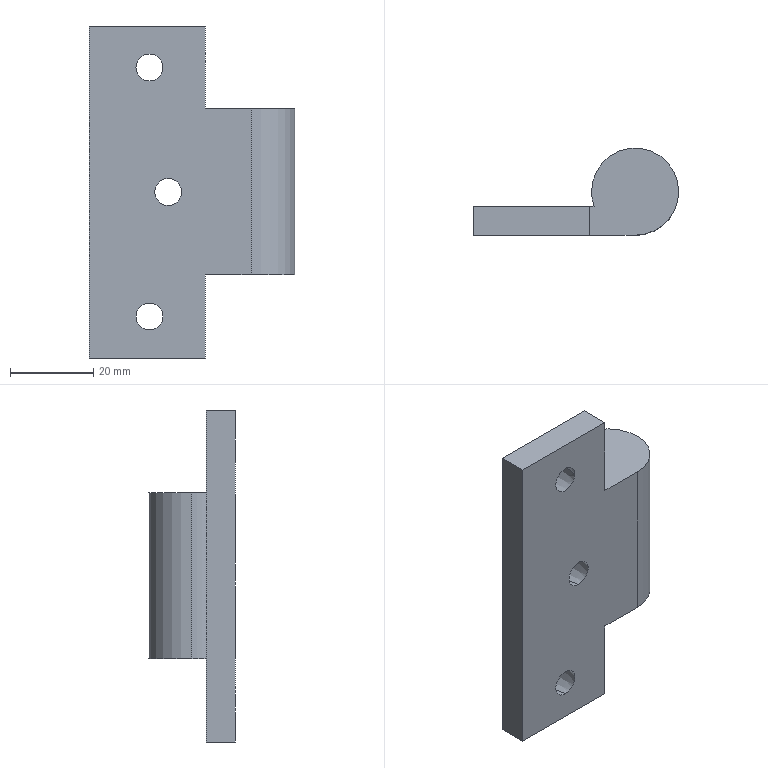Part | SolidWorks | features BaseBody 1 | 1 solid | 18 faces | box 49.5 x 21 x 80 mm | volume 29616 mm3 | plane 9 | cone 6 | cylinder 3 | commonest cylinder face diameters 21 x3
STEP:
#1=CARTESIAN_POINT('',(-10.5,0.,-20.));
#2=VERTEX_POINT('',#1);
#3=CARTESIAN_POINT('',(10.5,0.,-20.));
#4=VERTEX_POINT('',#3);
#5=CARTESIAN_POINT('',(0.,0.,-20.));
#6=DIRECTION('',(0.,0.,-1.));
#7=DIRECTION('',(1.,0.,0.));
#8=AXIS2_PLACEMENT_3D('',#5,#6,#7);
#9=CIRCLE('',#8,10.5);
#10=EDGE_CURVE('',#2,#4,#9,.T.);
#11=ORIENTED_EDGE('',*,*,#10,.F.);
#12=CARTESIAN_POINT('',(-10.5,0.,20.));
#13=VERTEX_POINT('',#12);
#14=CARTESIAN_POINT('',(-10.5,0.,40.));
#15=DIRECTION('',(0.,0.,1.));
#16=VECTOR('',#15,1000.);
#17=LINE('',#14,#16);
#18=EDGE_CURVE('',#2,#13,#17,.T.);
#19=ORIENTED_EDGE('',*,*,#18,.T.);
#20=CARTESIAN_POINT('',(10.5,0.,20.));
#21=VERTEX_POINT('',#20);
#22=CARTESIAN_POINT('',(0.,0.,20.));
#23=DIRECTION('',(0.,0.,1.));
#24=DIRECTION('',(1.,0.,0.));
#25=AXIS2_PLACEMENT_3D('',#22,#23,#24);
#26=CIRCLE('',#25,10.5);
#27=EDGE_CURVE('',#21,#13,#26,.T.);
#28=ORIENTED_EDGE('',*,*,#27,.F.);
#29=CARTESIAN_POINT('',(10.5,0.,40.));
#30=DIRECTION('',(0.,0.,1.));
#31=VECTOR('',#30,1000.);
#32=LINE('',#29,#31);
#33=EDGE_CURVE('',#4,#21,#32,.T.);
#34=ORIENTED_EDGE('',*,*,#33,.F.);
#35=EDGE_LOOP('',(#11,#19,#28,#34));
#36=FACE_OUTER_BOUND('',#35,.T.);
#37=CARTESIAN_POINT('',(0.,0.,40.));
#38=DIRECTION('',(0.,0.,1.));
#39=DIRECTION('',(1.,0.,0.));
#40=AXIS2_PLACEMENT_3D('',#37,#38,#39);
#41=CYLINDRICAL_SURFACE('',#40,10.5);
#42=ADVANCED_FACE('',(#36),#41,.T.);
#43=CARTESIAN_POINT('',(0.,-10.5,-20.));
#44=VERTEX_POINT('',#43);
#45=CARTESIAN_POINT('',(0.,0.,-20.));
#46=DIRECTION('',(0.,0.,-1.));
#47=DIRECTION('',(1.,0.,0.));
#48=AXIS2_PLACEMENT_3D('',#45,#46,#47);
#49=CIRCLE('',#48,10.5);
#50=EDGE_CURVE('',#4,#44,#49,.T.);
#51=ORIENTED_EDGE('',*,*,#50,.F.);
#52=ORIENTED_EDGE('',*,*,#33,.T.);
#53=CARTESIAN_POINT('',(0.,-10.5,20.));
#54=VERTEX_POINT('',#53);
#55=CARTESIAN_POINT('',(0.,0.,20.));
#56=DIRECTION('',(0.,0.,1.));
#57=DIRECTION('',(1.,0.,0.));
#58=AXIS2_PLACEMENT_3D('',#55,#56,#57);
#59=CIRCLE('',#58,10.5);
#60=EDGE_CURVE('',#54,#21,#59,.T.);
#61=ORIENTED_EDGE('',*,*,#60,.F.);
#62=CARTESIAN_POINT('',(0.,-10.5,40.));
#63=DIRECTION('',(0.,0.,-1.));
#64=VECTOR('',#63,1000.);
#65=LINE('',#62,#64);
#66=EDGE_CURVE('',#54,#44,#65,.T.);
#67=ORIENTED_EDGE('',*,*,#66,.T.);
#68=EDGE_LOOP('',(#51,#52,#61,#67));
#69=FACE_OUTER_BOUND('',#68,.T.);
#70=CARTESIAN_POINT('',(0.,0.,40.));
#71=DIRECTION('',(0.,0.,1.));
#72=DIRECTION('',(1.,0.,0.));
#73=AXIS2_PLACEMENT_3D('',#70,#71,#72);
#74=CYLINDRICAL_SURFACE('',#73,10.5);
#75=ADVANCED_FACE('',(#69),#74,.T.);
#76=CARTESIAN_POINT('',(-20.,-10.5,3.25));
#77=VERTEX_POINT('',#76);
#78=CARTESIAN_POINT('',(-20.,-10.5,-3.25));
#79=VERTEX_POINT('',#78);
#80=CARTESIAN_POINT('',(-20.,-10.5,0.));
#81=DIRECTION('',(0.,-1.,0.));
#82=DIRECTION('',(0.,0.,1.));
#83=AXIS2_PLACEMENT_3D('',#80,#81,#82);
#84=CIRCLE('',#83,3.25);
#85=EDGE_CURVE('',#77,#79,#84,.T.);
#86=ORIENTED_EDGE('',*,*,#85,.T.);
#87=CARTESIAN_POINT('',(-20.,-3.5,-4.417));
#88=VERTEX_POINT('',#87);
#89=CARTESIAN_POINT('',(-20.,-3.5,-4.417));
#90=DIRECTION('',(0.,0.9864,-0.1644));
#91=VECTOR('',#90,1000.);
#92=LINE('',#89,#91);
#93=EDGE_CURVE('',#79,#88,#92,.T.);
#94=ORIENTED_EDGE('',*,*,#93,.T.);
#95=CARTESIAN_POINT('',(-20.,-3.5,4.417));
#96=VERTEX_POINT('',#95);
#97=CARTESIAN_POINT('',(-20.,-3.5,0.));
#98=DIRECTION('',(0.,-1.,0.));
#99=DIRECTION('',(0.,0.,1.));
#100=AXIS2_PLACEMENT_3D('',#97,#98,#99);
#101=CIRCLE('',#100,4.417);
#102=EDGE_CURVE('',#96,#88,#101,.T.);
#103=ORIENTED_EDGE('',*,*,#102,.F.);
#104=CARTESIAN_POINT('',(-20.,-3.5,4.417));
#105=DIRECTION('',(0.,0.9864,0.1644));
#106=VECTOR('',#105,1000.);
#107=LINE('',#104,#106);
#108=EDGE_CURVE('',#77,#96,#107,.T.);
#109=ORIENTED_EDGE('',*,*,#108,.F.);
#110=EDGE_LOOP('',(#86,#94,#103,#109));
#111=FACE_OUTER_BOUND('',#110,.T.);
#112=CARTESIAN_POINT('',(-20.,-3.5,0.));
#113=DIRECTION('',(0.,1.,0.));
#114=DIRECTION('',(0.,0.,1.));
#115=AXIS2_PLACEMENT_3D('',#112,#113,#114);
#116=CONICAL_SURFACE('',#115,4.417,0.1651);
#117=ADVANCED_FACE('',(#111),#116,.F.);
#118=CARTESIAN_POINT('',(-24.5,-10.5,-26.75));
#119=VERTEX_POINT('',#118);
#120=CARTESIAN_POINT('',(-24.5,-10.5,-33.25));
#121=VERTEX_POINT('',#120);
#122=CARTESIAN_POINT('',(-24.5,-10.5,-30.));
#123=DIRECTION('',(0.,-1.,0.));
#124=DIRECTION('',(0.,0.,1.));
#125=AXIS2_PLACEMENT_3D('',#122,#123,#124);
#126=CIRCLE('',#125,3.25);
#127=EDGE_CURVE('',#119,#121,#126,.T.);
#128=ORIENTED_EDGE('',*,*,#127,.T.);
#129=CARTESIAN_POINT('',(-24.5,-3.5,-34.417));
#130=VERTEX_POINT('',#129);
#131=CARTESIAN_POINT('',(-24.5,-3.5,-34.417));
#132=DIRECTION('',(0.,0.9864,-0.1644));
#133=VECTOR('',#132,1000.);
#134=LINE('',#131,#133);
#135=EDGE_CURVE('',#121,#130,#134,.T.);
#136=ORIENTED_EDGE('',*,*,#135,.T.);
#137=CARTESIAN_POINT('',(-24.5,-3.5,-25.583));
#138=VERTEX_POINT('',#137);
#139=CARTESIAN_POINT('',(-24.5,-3.5,-30.));
#140=DIRECTION('',(0.,-1.,0.));
#141=DIRECTION('',(0.,0.,1.));
#142=AXIS2_PLACEMENT_3D('',#139,#140,#141);
#143=CIRCLE('',#142,4.417);
#144=EDGE_CURVE('',#138,#130,#143,.T.);
#145=ORIENTED_EDGE('',*,*,#144,.F.);
#146=CARTESIAN_POINT('',(-24.5,-3.5,-25.583));
#147=DIRECTION('',(0.,0.9864,0.1644));
#148=VECTOR('',#147,1000.);
#149=LINE('',#146,#148);
#150=EDGE_CURVE('',#119,#138,#149,.T.);
#151=ORIENTED_EDGE('',*,*,#150,.F.);
#152=EDGE_LOOP('',(#128,#136,#145,#151));
#153=FACE_OUTER_BOUND('',#152,.T.);
#154=CARTESIAN_POINT('',(-24.5,-3.5,-30.));
#155=DIRECTION('',(0.,1.,0.));
#156=DIRECTION('',(0.,0.,1.));
#157=AXIS2_PLACEMENT_3D('',#154,#155,#156);
#158=CONICAL_SURFACE('',#157,4.417,0.1651);
#159=ADVANCED_FACE('',(#153),#158,.F.);
#160=CARTESIAN_POINT('',(-27.75,-10.5,30.));
#161=VERTEX_POINT('',#160);
#162=CARTESIAN_POINT('',(-21.25,-10.5,30.));
#163=VERTEX_POINT('',#162);
#164=CARTESIAN_POINT('',(-24.5,-10.5,30.));
#165=DIRECTION('',(0.,-1.,0.));
#166=DIRECTION('',(-1.,0.,0.));
#167=AXIS2_PLACEMENT_3D('',#164,#165,#166);
#168=CIRCLE('',#167,3.25);
#169=EDGE_CURVE('',#161,#163,#168,.T.);
#170=ORIENTED_EDGE('',*,*,#169,.T.);
#171=CARTESIAN_POINT('',(-20.083,-3.5,30.));
#172=VERTEX_POINT('',#171);
#173=CARTESIAN_POINT('',(-20.083,-3.5,30.));
#174=DIRECTION('',(0.1644,0.9864,0.));
#175=VECTOR('',#174,1000.);
#176=LINE('',#173,#175);
#177=EDGE_CURVE('',#163,#172,#176,.T.);
#178=ORIENTED_EDGE('',*,*,#177,.T.);
#179=CARTESIAN_POINT('',(-28.917,-3.5,30.));
#180=VERTEX_POINT('',#179);
#181=CARTESIAN_POINT('',(-24.5,-3.5,30.));
#182=DIRECTION('',(0.,-1.,0.));
#183=DIRECTION('',(-1.,0.,0.));
#184=AXIS2_PLACEMENT_3D('',#181,#182,#183);
#185=CIRCLE('',#184,4.417);
#186=EDGE_CURVE('',#180,#172,#185,.T.);
#187=ORIENTED_EDGE('',*,*,#186,.F.);
#188=CARTESIAN_POINT('',(-28.917,-3.5,30.));
#189=DIRECTION('',(-0.1644,0.9864,0.));
#190=VECTOR('',#189,1000.);
#191=LINE('',#188,#190);
#192=EDGE_CURVE('',#161,#180,#191,.T.);
#193=ORIENTED_EDGE('',*,*,#192,.F.);
#194=EDGE_LOOP('',(#170,#178,#187,#193));
#195=FACE_OUTER_BOUND('',#194,.T.);
#196=CARTESIAN_POINT('',(-24.5,-3.5,30.));
#197=DIRECTION('',(0.,1.,0.));
#198=DIRECTION('',(-1.,0.,0.));
#199=AXIS2_PLACEMENT_3D('',#196,#197,#198);
#200=CONICAL_SURFACE('',#199,4.417,0.1651);
#201=ADVANCED_FACE('',(#195),#200,.F.);
#202=CARTESIAN_POINT('',(-11.,-10.5,40.));
#203=VERTEX_POINT('',#202);
#204=CARTESIAN_POINT('',(-11.,-10.5,20.));
#205=VERTEX_POINT('',#204);
#206=CARTESIAN_POINT('',(-11.,-10.5,40.));
#207=DIRECTION('',(0.,0.,-1.));
#208=VECTOR('',#207,1000.);
#209=LINE('',#206,#208);
#210=EDGE_CURVE('',#203,#205,#209,.T.);
#211=ORIENTED_EDGE('',*,*,#210,.F.);
#212=CARTESIAN_POINT('',(-39.,-10.5,40.));
#213=VERTEX_POINT('',#212);
#214=CARTESIAN_POINT('',(-39.,-10.5,40.));
#215=DIRECTION('',(1.,0.,0.));
#216=VECTOR('',#215,1000.);
#217=LINE('',#214,#216);
#218=EDGE_CURVE('',#213,#203,#217,.T.);
#219=ORIENTED_EDGE('',*,*,#218,.F.);
#220=CARTESIAN_POINT('',(-39.,-10.5,-40.));
#221=VERTEX_POINT('',#220);
#222=CARTESIAN_POINT('',(-39.,-10.5,40.));
#223=DIRECTION('',(0.,0.,1.));
#224=VECTOR('',#223,1000.);
#225=LINE('',#222,#224);
#226=EDGE_CURVE('',#221,#213,#225,.T.);
#227=ORIENTED_EDGE('',*,*,#226,.F.);
#228=CARTESIAN_POINT('',(-11.,-10.5,-40.));
#229=VERTEX_POINT('',#228);
#230=CARTESIAN_POINT('',(-39.,-10.5,-40.));
#231=DIRECTION('',(-1.,0.,0.));
#232=VECTOR('',#231,1000.);
#233=LINE('',#230,#232);
#234=EDGE_CURVE('',#229,#221,#233,.T.);
#235=ORIENTED_EDGE('',*,*,#234,.F.);
#236=CARTESIAN_POINT('',(-11.,-10.5,-20.));
#237=VERTEX_POINT('',#236);
#238=CARTESIAN_POINT('',(-11.,-10.5,40.));
#239=DIRECTION('',(0.,0.,-1.));
#240=VECTOR('',#239,1000.);
#241=LINE('',#238,#240);
#242=EDGE_CURVE('',#237,#229,#241,.T.);
#243=ORIENTED_EDGE('',*,*,#242,.F.);
#244=CARTESIAN_POINT('',(-39.,-10.5,-20.));
#245=DIRECTION('',(-1.,0.,0.));
#246=VECTOR('',#245,1000.);
#247=LINE('',#244,#246);
#248=EDGE_CURVE('',#44,#237,#247,.T.);
#249=ORIENTED_EDGE('',*,*,#248,.F.);
#250=ORIENTED_EDGE('',*,*,#66,.F.);
#251=CARTESIAN_POINT('',(-39.,-10.5,20.));
#252=DIRECTION('',(1.,0.,0.));
#253=VECTOR('',#252,1000.);
#254=LINE('',#251,#253);
#255=EDGE_CURVE('',#205,#54,#254,.T.);
#256=ORIENTED_EDGE('',*,*,#255,.F.);
#257=EDGE_LOOP('',(#211,#219,#227,#235,#243,#249,#250,#256));
#258=FACE_OUTER_BOUND('',#257,.T.);
#259=ORIENTED_EDGE('',*,*,#85,.F.);
#260=CARTESIAN_POINT('',(-20.,-10.5,0.));
#261=DIRECTION('',(0.,-1.,0.));
#262=DIRECTION('',(0.,0.,1.));
#263=AXIS2_PLACEMENT_3D('',#260,#261,#262);
#264=CIRCLE('',#263,3.25);
#265=EDGE_CURVE('',#79,#77,#264,.T.);
#266=ORIENTED_EDGE('',*,*,#265,.F.);
#267=EDGE_LOOP('',(#259,#266));
#268=FACE_BOUND('',#267,.T.);
#269=ORIENTED_EDGE('',*,*,#127,.F.);
#270=CARTESIAN_POINT('',(-24.5,-10.5,-30.));
#271=DIRECTION('',(0.,-1.,0.));
#272=DIRECTION('',(0.,0.,1.));
#273=AXIS2_PLACEMENT_3D('',#270,#271,#272);
#274=CIRCLE('',#273,3.25);
#275=EDGE_CURVE('',#121,#119,#274,.T.);
#276=ORIENTED_EDGE('',*,*,#275,.F.);
#277=EDGE_LOOP('',(#269,#276));
#278=FACE_BOUND('',#277,.T.);
#279=ORIENTED_EDGE('',*,*,#169,.F.);
#280=CARTESIAN_POINT('',(-24.5,-10.5,30.));
#281=DIRECTION('',(0.,-1.,0.));
#282=DIRECTION('',(-1.,0.,0.));
#283=AXIS2_PLACEMENT_3D('',#280,#281,#282);
#284=CIRCLE('',#283,3.25);
#285=EDGE_CURVE('',#163,#161,#284,.T.);
#286=ORIENTED_EDGE('',*,*,#285,.F.);
#287=EDGE_LOOP('',(#279,#286));
#288=FACE_BOUND('',#287,.T.);
#289=CARTESIAN_POINT('',(-39.,-10.5,40.));
#290=DIRECTION('',(0.,1.,0.));
#291=DIRECTION('',(0.,0.,1.));
#292=AXIS2_PLACEMENT_3D('',#289,#290,#291);
#293=PLANE('',#292);
#294=ADVANCED_FACE('',(#258,#268,#278,#288),#293,.F.);
#295=ORIENTED_EDGE('',*,*,#255,.T.);
#296=ORIENTED_EDGE('',*,*,#60,.T.);
#297=ORIENTED_EDGE('',*,*,#27,.T.);
#298=CARTESIAN_POINT('',(-9.899,-3.5,20.));
#299=VERTEX_POINT('',#298);
#300=CARTESIAN_POINT('',(0.,0.,20.));
#301=DIRECTION('',(0.,0.,1.));
#302=DIRECTION('',(1.,0.,0.));
#303=AXIS2_PLACEMENT_3D('',#300,#301,#302);
#304=CIRCLE('',#303,10.5);
#305=EDGE_CURVE('',#13,#299,#304,.T.);
#306=ORIENTED_EDGE('',*,*,#305,.T.);
#307=CARTESIAN_POINT('',(-11.,-3.5,20.));
#308=VERTEX_POINT('',#307);
#309=CARTESIAN_POINT('',(-9.899,-3.5,20.));
#310=DIRECTION('',(-1.,0.,0.));
#311=VECTOR('',#310,1000.);
#312=LINE('',#309,#311);
#313=EDGE_CURVE('',#299,#308,#312,.T.);
#314=ORIENTED_EDGE('',*,*,#313,.T.);
#315=CARTESIAN_POINT('',(-11.,19.,20.));
#316=DIRECTION('',(0.,-1.,0.));
#317=VECTOR('',#316,1000.);
#318=LINE('',#315,#317);
#319=EDGE_CURVE('',#308,#205,#318,.T.);
#320=ORIENTED_EDGE('',*,*,#319,.T.);
#321=EDGE_LOOP('',(#295,#296,#297,#306,#314,#320));
#322=FACE_OUTER_BOUND('',#321,.T.);
#323=CARTESIAN_POINT('',(11.,19.,20.));
#324=DIRECTION('',(0.,0.,1.));
#325=DIRECTION('',(1.,0.,0.));
#326=AXIS2_PLACEMENT_3D('',#323,#324,#325);
#327=PLANE('',#326);
#328=ADVANCED_FACE('',(#322),#327,.T.);
#329=ORIENTED_EDGE('',*,*,#210,.T.);
#330=ORIENTED_EDGE('',*,*,#319,.F.);
#331=CARTESIAN_POINT('',(-11.,-3.5,40.));
#332=VERTEX_POINT('',#331);
#333=CARTESIAN_POINT('',(-11.,-3.5,20.));
#334=DIRECTION('',(0.,0.,1.));
#335=VECTOR('',#334,1000.);
#336=LINE('',#333,#335);
#337=EDGE_CURVE('',#308,#332,#336,.T.);
#338=ORIENTED_EDGE('',*,*,#337,.T.);
#339=CARTESIAN_POINT('',(-11.,19.,40.));
#340=DIRECTION('',(0.,-1.,0.));
#341=VECTOR('',#340,1000.);
#342=LINE('',#339,#341);
#343=EDGE_CURVE('',#332,#203,#342,.T.);
#344=ORIENTED_EDGE('',*,*,#343,.T.);
#345=EDGE_LOOP('',(#329,#330,#338,#344));
#346=FACE_OUTER_BOUND('',#345,.T.);
#347=CARTESIAN_POINT('',(-11.,19.,20.));
#348=DIRECTION('',(1.,0.,0.));
#349=DIRECTION('',(0.,0.,-1.));
#350=AXIS2_PLACEMENT_3D('',#347,#348,#349);
#351=PLANE('',#350);
#352=ADVANCED_FACE('',(#346),#351,.T.);
#353=CARTESIAN_POINT('',(-39.,-3.5,40.));
#354=VERTEX_POINT('',#353);
#355=CARTESIAN_POINT('',(0.,-3.5,40.));
#356=DIRECTION('',(-1.,0.,0.));
#357=VECTOR('',#356,1000.);
#358=LINE('',#355,#357);
#359=EDGE_CURVE('',#332,#354,#358,.T.);
#360=ORIENTED_EDGE('',*,*,#359,.T.);
#361=CARTESIAN_POINT('',(-39.,0.,40.));
#362=DIRECTION('',(0.,-1.,0.));
#363=VECTOR('',#362,1000.);
#364=LINE('',#361,#363);
#365=EDGE_CURVE('',#354,#213,#364,.T.);
#366=ORIENTED_EDGE('',*,*,#365,.T.);
#367=ORIENTED_EDGE('',*,*,#218,.T.);
#368=ORIENTED_EDGE('',*,*,#343,.F.);
#369=EDGE_LOOP('',(#360,#366,#367,#368));
#370=FACE_OUTER_BOUND('',#369,.T.);
#371=CARTESIAN_POINT('',(0.,0.,40.));
#372=DIRECTION('',(0.,0.,1.));
#373=DIRECTION('',(1.,0.,0.));
#374=AXIS2_PLACEMENT_3D('',#371,#372,#373);
#375=PLANE('',#374);
#376=ADVANCED_FACE('',(#370),#375,.T.);
#377=ORIENTED_EDGE('',*,*,#226,.T.);
#378=ORIENTED_EDGE('',*,*,#365,.F.);
#379=CARTESIAN_POINT('',(-39.,-3.5,-40.));
#380=VERTEX_POINT('',#379);
#381=CARTESIAN_POINT('',(-39.,-3.5,40.));
#382=DIRECTION('',(0.,0.,1.));
#383=VECTOR('',#382,1000.);
#384=LINE('',#381,#383);
#385=EDGE_CURVE('',#380,#354,#384,.T.);
#386=ORIENTED_EDGE('',*,*,#385,.F.);
#387=CARTESIAN_POINT('',(-39.,-3.5,-40.));
#388=DIRECTION('',(0.,1.,0.));
#389=VECTOR('',#388,1000.);
#390=LINE('',#387,#389);
#391=EDGE_CURVE('',#221,#380,#390,.T.);
#392=ORIENTED_EDGE('',*,*,#391,.F.);
#393=EDGE_LOOP('',(#377,#378,#386,#392));
#394=FACE_OUTER_BOUND('',#393,.T.);
#395=CARTESIAN_POINT('',(-39.,-3.5,40.));
#396=DIRECTION('',(1.,0.,0.));
#397=DIRECTION('',(0.,0.,-1.));
#398=AXIS2_PLACEMENT_3D('',#395,#396,#397);
#399=PLANE('',#398);
#400=ADVANCED_FACE('',(#394),#399,.F.);
#401=ORIENTED_EDGE('',*,*,#234,.T.);
#402=ORIENTED_EDGE('',*,*,#391,.T.);
#403=CARTESIAN_POINT('',(-11.,-3.5,-40.));
#404=VERTEX_POINT('',#403);
#405=CARTESIAN_POINT('',(0.,-3.5,-40.));
#406=DIRECTION('',(-1.,0.,0.));
#407=VECTOR('',#406,1000.);
#408=LINE('',#405,#407);
#409=EDGE_CURVE('',#404,#380,#408,.T.);
#410=ORIENTED_EDGE('',*,*,#409,.F.);
#411=CARTESIAN_POINT('',(-11.,0.,-40.));
#412=DIRECTION('',(0.,1.,0.));
#413=VECTOR('',#412,1000.);
#414=LINE('',#411,#413);
#415=EDGE_CURVE('',#229,#404,#414,.T.);
#416=ORIENTED_EDGE('',*,*,#415,.F.);
#417=EDGE_LOOP('',(#401,#402,#410,#416));
#418=FACE_OUTER_BOUND('',#417,.T.);
#419=CARTESIAN_POINT('',(0.,0.,-40.));
#420=DIRECTION('',(0.,0.,1.));
#421=DIRECTION('',(1.,0.,0.));
#422=AXIS2_PLACEMENT_3D('',#419,#420,#421);
#423=PLANE('',#422);
#424=ADVANCED_FACE('',(#418),#423,.F.);
#425=ORIENTED_EDGE('',*,*,#242,.T.);
#426=ORIENTED_EDGE('',*,*,#415,.T.);
#427=CARTESIAN_POINT('',(-11.,-3.5,-20.));
#428=VERTEX_POINT('',#427);
#429=CARTESIAN_POINT('',(-11.,-3.5,-40.));
#430=DIRECTION('',(0.,0.,1.));
#431=VECTOR('',#430,1000.);
#432=LINE('',#429,#431);
#433=EDGE_CURVE('',#404,#428,#432,.T.);
#434=ORIENTED_EDGE('',*,*,#433,.T.);
#435=CARTESIAN_POINT('',(-11.,19.,-20.));
#436=DIRECTION('',(0.,-1.,0.));
#437=VECTOR('',#436,1000.);
#438=LINE('',#435,#437);
#439=EDGE_CURVE('',#428,#237,#438,.T.);
#440=ORIENTED_EDGE('',*,*,#439,.T.);
#441=EDGE_LOOP('',(#425,#426,#434,#440));
#442=FACE_OUTER_BOUND('',#441,.T.);
#443=CARTESIAN_POINT('',(-11.,19.,-40.));
#444=DIRECTION('',(1.,0.,0.));
#445=DIRECTION('',(0.,0.,-1.));
#446=AXIS2_PLACEMENT_3D('',#443,#444,#445);
#447=PLANE('',#446);
#448=ADVANCED_FACE('',(#442),#447,.T.);
#449=ORIENTED_EDGE('',*,*,#248,.T.);
#450=ORIENTED_EDGE('',*,*,#439,.F.);
#451=CARTESIAN_POINT('',(-9.899,-3.5,-20.));
#452=VERTEX_POINT('',#451);
#453=CARTESIAN_POINT('',(-11.,-3.5,-20.));
#454=DIRECTION('',(1.,0.,0.));
#455=VECTOR('',#454,1000.);
#456=LINE('',#453,#455);
#457=EDGE_CURVE('',#428,#452,#456,.T.);
#458=ORIENTED_EDGE('',*,*,#457,.T.);
#459=CARTESIAN_POINT('',(0.,0.,-20.));
#460=DIRECTION('',(0.,0.,-1.));
#461=DIRECTION('',(1.,0.,0.));
#462=AXIS2_PLACEMENT_3D('',#459,#460,#461);
#463=CIRCLE('',#462,10.5);
#464=EDGE_CURVE('',#452,#2,#463,.T.);
#465=ORIENTED_EDGE('',*,*,#464,.T.);
#466=ORIENTED_EDGE('',*,*,#10,.T.);
#467=ORIENTED_EDGE('',*,*,#50,.T.);
#468=EDGE_LOOP('',(#449,#450,#458,#465,#466,#467));
#469=FACE_OUTER_BOUND('',#468,.T.);
#470=CARTESIAN_POINT('',(-11.,19.,-20.));
#471=DIRECTION('',(0.,0.,-1.));
#472=DIRECTION('',(-1.,0.,0.));
#473=AXIS2_PLACEMENT_3D('',#470,#471,#472);
#474=PLANE('',#473);
#475=ADVANCED_FACE('',(#469),#474,.T.);
#476=ORIENTED_EDGE('',*,*,#18,.F.);
#477=ORIENTED_EDGE('',*,*,#464,.F.);
#478=CARTESIAN_POINT('',(-9.899,-3.5,40.));
#479=DIRECTION('',(0.,0.,1.));
#480=VECTOR('',#479,1000.);
#481=LINE('',#478,#480);
#482=EDGE_CURVE('',#452,#299,#481,.T.);
#483=ORIENTED_EDGE('',*,*,#482,.T.);
#484=ORIENTED_EDGE('',*,*,#305,.F.);
#485=EDGE_LOOP('',(#476,#477,#483,#484));
#486=FACE_OUTER_BOUND('',#485,.T.);
#487=CARTESIAN_POINT('',(0.,0.,40.));
#488=DIRECTION('',(0.,0.,1.));
#489=DIRECTION('',(1.,0.,0.));
#490=AXIS2_PLACEMENT_3D('',#487,#488,#489);
#491=CYLINDRICAL_SURFACE('',#490,10.5);
#492=ADVANCED_FACE('',(#486),#491,.T.);
#493=ORIENTED_EDGE('',*,*,#93,.F.);
#494=ORIENTED_EDGE('',*,*,#265,.T.);
#495=ORIENTED_EDGE('',*,*,#108,.T.);
#496=CARTESIAN_POINT('',(-20.,-3.5,0.));
#497=DIRECTION('',(0.,-1.,0.));
#498=DIRECTION('',(0.,0.,1.));
#499=AXIS2_PLACEMENT_3D('',#496,#497,#498);
#500=CIRCLE('',#499,4.417);
#501=EDGE_CURVE('',#88,#96,#500,.T.);
#502=ORIENTED_EDGE('',*,*,#501,.F.);
#503=EDGE_LOOP('',(#493,#494,#495,#502));
#504=FACE_OUTER_BOUND('',#503,.T.);
#505=CARTESIAN_POINT('',(-20.,-3.5,0.));
#506=DIRECTION('',(0.,1.,0.));
#507=DIRECTION('',(0.,0.,1.));
#508=AXIS2_PLACEMENT_3D('',#505,#506,#507);
#509=CONICAL_SURFACE('',#508,4.417,0.1651);
#510=ADVANCED_FACE('',(#504),#509,.F.);
#511=ORIENTED_EDGE('',*,*,#135,.F.);
#512=ORIENTED_EDGE('',*,*,#275,.T.);
#513=ORIENTED_EDGE('',*,*,#150,.T.);
#514=CARTESIAN_POINT('',(-24.5,-3.5,-30.));
#515=DIRECTION('',(0.,-1.,0.));
#516=DIRECTION('',(0.,0.,1.));
#517=AXIS2_PLACEMENT_3D('',#514,#515,#516);
#518=CIRCLE('',#517,4.417);
#519=EDGE_CURVE('',#130,#138,#518,.T.);
#520=ORIENTED_EDGE('',*,*,#519,.F.);
#521=EDGE_LOOP('',(#511,#512,#513,#520));
#522=FACE_OUTER_BOUND('',#521,.T.);
#523=CARTESIAN_POINT('',(-24.5,-3.5,-30.));
#524=DIRECTION('',(0.,1.,0.));
#525=DIRECTION('',(0.,0.,1.));
#526=AXIS2_PLACEMENT_3D('',#523,#524,#525);
#527=CONICAL_SURFACE('',#526,4.417,0.1651);
#528=ADVANCED_FACE('',(#522),#527,.F.);
#529=ORIENTED_EDGE('',*,*,#177,.F.);
#530=ORIENTED_EDGE('',*,*,#285,.T.);
#531=ORIENTED_EDGE('',*,*,#192,.T.);
#532=CARTESIAN_POINT('',(-24.5,-3.5,30.));
#533=DIRECTION('',(0.,-1.,0.));
#534=DIRECTION('',(-1.,0.,0.));
#535=AXIS2_PLACEMENT_3D('',#532,#533,#534);
#536=CIRCLE('',#535,4.417);
#537=EDGE_CURVE('',#172,#180,#536,.T.);
#538=ORIENTED_EDGE('',*,*,#537,.F.);
#539=EDGE_LOOP('',(#529,#530,#531,#538));
#540=FACE_OUTER_BOUND('',#539,.T.);
#541=CARTESIAN_POINT('',(-24.5,-3.5,30.));
#542=DIRECTION('',(0.,1.,0.));
#543=DIRECTION('',(-1.,0.,0.));
#544=AXIS2_PLACEMENT_3D('',#541,#542,#543);
#545=CONICAL_SURFACE('',#544,4.417,0.1651);
#546=ADVANCED_FACE('',(#540),#545,.F.);
#547=ORIENTED_EDGE('',*,*,#482,.F.);
#548=ORIENTED_EDGE('',*,*,#457,.F.);
#549=ORIENTED_EDGE('',*,*,#433,.F.);
#550=ORIENTED_EDGE('',*,*,#409,.T.);
#551=ORIENTED_EDGE('',*,*,#385,.T.);
#552=ORIENTED_EDGE('',*,*,#359,.F.);
#553=ORIENTED_EDGE('',*,*,#337,.F.);
#554=ORIENTED_EDGE('',*,*,#313,.F.);
#555=EDGE_LOOP('',(#547,#548,#549,#550,#551,#552,#553,#554));
#556=FACE_OUTER_BOUND('',#555,.T.);
#557=ORIENTED_EDGE('',*,*,#102,.T.);
#558=ORIENTED_EDGE('',*,*,#501,.T.);
#559=EDGE_LOOP('',(#557,#558));
#560=FACE_BOUND('',#559,.T.);
#561=ORIENTED_EDGE('',*,*,#144,.T.);
#562=ORIENTED_EDGE('',*,*,#519,.T.);
#563=EDGE_LOOP('',(#561,#562));
#564=FACE_BOUND('',#563,.T.);
#565=ORIENTED_EDGE('',*,*,#186,.T.);
#566=ORIENTED_EDGE('',*,*,#537,.T.);
#567=EDGE_LOOP('',(#565,#566));
#568=FACE_BOUND('',#567,.T.);
#569=CARTESIAN_POINT('',(-9.899,-3.5,40.));
#570=DIRECTION('',(0.,-1.,0.));
#571=DIRECTION('',(0.,0.,-1.));
#572=AXIS2_PLACEMENT_3D('',#569,#570,#571);
#573=PLANE('',#572);
#574=ADVANCED_FACE('',(#556,#560,#564,#568),#573,.F.);
#575=CLOSED_SHELL('',(#42,#75,#117,#159,#201,#294,#328,#352,#376,#400,#424,#448,#475,#492,#510,#528,#546,#574));
#576=MANIFOLD_SOLID_BREP('',#575);
#577=CARTESIAN_POINT('',(0.,0.,0.));
#578=DIRECTION('',(0.,0.,1.));
#579=DIRECTION('',(1.,0.,0.));
#580=AXIS2_PLACEMENT_3D('',#577,#578,#579);
#581=(LENGTH_UNIT()NAMED_UNIT(*)SI_UNIT(.MILLI.,.METRE.));
#582=UNCERTAINTY_MEASURE_WITH_UNIT(LENGTH_MEASURE(0.00001),#581,'','');
#583=(NAMED_UNIT(*)PLANE_ANGLE_UNIT()SI_UNIT($,.RADIAN.));
#584=(NAMED_UNIT(*)SI_UNIT($,.STERADIAN.)SOLID_ANGLE_UNIT());
#585=(GEOMETRIC_REPRESENTATION_CONTEXT(3)GLOBAL_UNCERTAINTY_ASSIGNED_CONTEXT((#582))GLOBAL_UNIT_ASSIGNED_CONTEXT((#581,#583,#584))REPRESENTATION_CONTEXT('',''));
#586=ADVANCED_BREP_SHAPE_REPRESENTATION('',(#576,#580),#585);